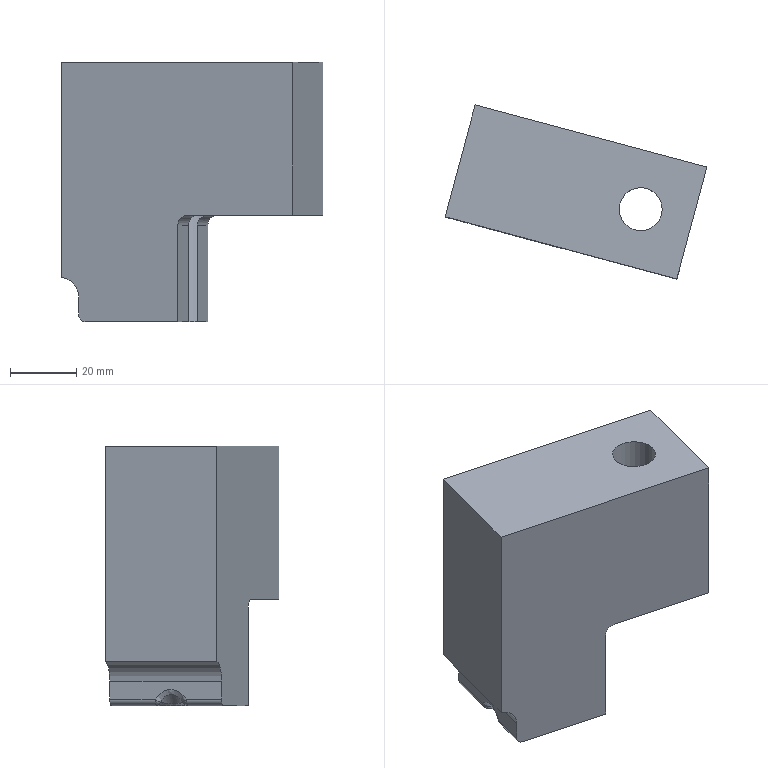Part | NX | features solid 2 | 1 solid | 27 faces | box 79.088 x 52.572 x 78.4 mm | volume 141118 mm3 | plane 12 | cylinder 10 | spline 4 | cone 1 | commonest cylinder face diameters 4 x2 6 x2 8.5 x1 10 x1 11 x1 12 x1
STEP:
#1=CARTESIAN_POINT('',(1214.961,-8.867,-0.02087));
#2=VERTEX_POINT('',#1);
#3=CARTESIAN_POINT('',(1214.961,-8.867,65.));
#4=VERTEX_POINT('',#3);
#5=CARTESIAN_POINT('',(1214.961,-8.867,86.));
#6=DIRECTION('',(0.,0.,1.));
#7=VECTOR('',#6,1000.);
#8=LINE('',#5,#7);
#9=EDGE_CURVE('',#2,#4,#8,.T.);
#10=ORIENTED_EDGE('',*,*,#9,.T.);
#11=CARTESIAN_POINT('',(1284.991,-27.632,65.));
#12=VERTEX_POINT('',#11);
#13=CARTESIAN_POINT('',(1303.344,-32.549,65.));
#14=DIRECTION('',(0.9659,-0.2588,0.));
#15=VECTOR('',#14,1000.);
#16=LINE('',#13,#15);
#17=EDGE_CURVE('',#4,#12,#16,.T.);
#18=ORIENTED_EDGE('',*,*,#17,.T.);
#19=CARTESIAN_POINT('',(1284.991,-27.632,18.75));
#20=VERTEX_POINT('',#19);
#21=CARTESIAN_POINT('',(1284.991,-27.632,142.6));
#22=DIRECTION('',(0.,0.,1.));
#23=VECTOR('',#22,1000.);
#24=LINE('',#21,#23);
#25=EDGE_CURVE('',#20,#12,#24,.T.);
#26=ORIENTED_EDGE('',*,*,#25,.F.);
#27=CARTESIAN_POINT('',(1253.115,-19.091,18.75));
#28=VERTEX_POINT('',#27);
#29=CARTESIAN_POINT('',(1303.344,-32.549,18.75));
#30=DIRECTION('',(0.9659,-0.2588,0.));
#31=VECTOR('',#30,1000.);
#32=LINE('',#29,#31);
#33=EDGE_CURVE('',#20,#28,#32,.F.);
#34=ORIENTED_EDGE('',*,*,#33,.T.);
#35=CARTESIAN_POINT('',(1250.218,-18.314,15.75));
#36=VERTEX_POINT('',#35);
#37=CARTESIAN_POINT('',(1253.115,-19.091,15.75));
#38=DIRECTION('',(-0.2588,-0.9659,0.));
#39=DIRECTION('',(0.9659,-0.2588,0.));
#40=AXIS2_PLACEMENT_3D('',#37,#38,#39);
#41=CIRCLE('',#40,3.);
#42=EDGE_CURVE('',#36,#28,#41,.F.);
#43=ORIENTED_EDGE('',*,*,#42,.F.);
#44=CARTESIAN_POINT('',(1250.218,-18.314,-13.4));
#45=VERTEX_POINT('',#44);
#46=CARTESIAN_POINT('',(1250.218,-18.314,142.6));
#47=DIRECTION('',(0.,0.,1.));
#48=VECTOR('',#47,1000.);
#49=LINE('',#46,#48);
#50=EDGE_CURVE('',#45,#36,#49,.T.);
#51=ORIENTED_EDGE('',*,*,#50,.F.);
#52=CARTESIAN_POINT('',(1222.206,-10.808,-13.4));
#53=VERTEX_POINT('',#52);
#54=CARTESIAN_POINT('',(1303.344,-32.549,-13.4));
#55=DIRECTION('',(0.9659,-0.2588,0.));
#56=VECTOR('',#55,1000.);
#57=LINE('',#54,#56);
#58=EDGE_CURVE('',#45,#53,#57,.F.);
#59=ORIENTED_EDGE('',*,*,#58,.T.);
#60=CARTESIAN_POINT('',(1220.274,-10.291,-11.4));
#61=VERTEX_POINT('',#60);
#62=CARTESIAN_POINT('',(1222.206,-10.808,-11.4));
#63=DIRECTION('',(0.2588,0.9659,0.));
#64=DIRECTION('',(-0.9659,0.2588,0.));
#65=AXIS2_PLACEMENT_3D('',#62,#63,#64);
#66=CIRCLE('',#65,2.);
#67=EDGE_CURVE('',#61,#53,#66,.F.);
#68=ORIENTED_EDGE('',*,*,#67,.F.);
#69=CARTESIAN_POINT('',(1220.274,-10.291,-6.));
#70=VERTEX_POINT('',#69);
#71=CARTESIAN_POINT('',(1220.274,-10.291,0.));
#72=DIRECTION('',(0.,0.,1.));
#73=VECTOR('',#72,1000.);
#74=LINE('',#71,#73);
#75=EDGE_CURVE('',#70,#61,#74,.F.);
#76=ORIENTED_EDGE('',*,*,#75,.F.);
#77=CARTESIAN_POINT('',(1214.478,-8.738,-6.));
#78=DIRECTION('',(0.2588,0.9659,0.));
#79=DIRECTION('',(-0.9659,0.2588,0.));
#80=AXIS2_PLACEMENT_3D('',#77,#78,#79);
#81=CIRCLE('',#80,6.);
#82=EDGE_CURVE('',#2,#70,#81,.T.);
#83=ORIENTED_EDGE('',*,*,#82,.F.);
#84=EDGE_LOOP('',(#10,#18,#26,#34,#43,#51,#59,#68,#76,#83));
#85=FACE_BOUND('',#84,.T.);
#86=CARTESIAN_POINT('',(1303.344,-32.549,-6.));
#87=DIRECTION('',(0.2588,0.9659,0.));
#88=DIRECTION('',(-0.9659,0.2588,0.));
#89=AXIS2_PLACEMENT_3D('',#86,#87,#88);
#90=PLANE('',#89);
#91=ADVANCED_FACE('',(#85),#90,.T.);
#92=CARTESIAN_POINT('',(1205.903,-42.675,65.));
#93=VERTEX_POINT('',#92);
#94=CARTESIAN_POINT('',(1205.903,-42.675,-0.02087));
#95=VERTEX_POINT('',#94);
#96=CARTESIAN_POINT('',(1205.903,-42.675,181.6));
#97=DIRECTION('',(0.,0.,-1.));
#98=VECTOR('',#97,1000.);
#99=LINE('',#96,#98);
#100=EDGE_CURVE('',#93,#95,#99,.T.);
#101=ORIENTED_EDGE('',*,*,#100,.F.);
#102=CARTESIAN_POINT('',(1203.025,-53.415,65.));
#103=DIRECTION('',(0.2588,0.9659,0.));
#104=VECTOR('',#103,1000.);
#105=LINE('',#102,#104);
#106=EDGE_CURVE('',#93,#4,#105,.T.);
#107=ORIENTED_EDGE('',*,*,#106,.T.);
#108=ORIENTED_EDGE('',*,*,#9,.F.);
#109=CARTESIAN_POINT('',(1215.168,-8.097,-0.02087));
#110=DIRECTION('',(0.2588,0.9659,0.));
#111=VECTOR('',#110,1000.);
#112=LINE('',#109,#111);
#113=EDGE_CURVE('',#2,#95,#112,.F.);
#114=ORIENTED_EDGE('',*,*,#113,.T.);
#115=EDGE_LOOP('',(#101,#107,#108,#114));
#116=FACE_BOUND('',#115,.T.);
#117=CARTESIAN_POINT('',(1203.025,-53.415,86.));
#118=DIRECTION('',(-0.9659,0.2588,0.));
#119=DIRECTION('',(-0.2588,-0.9659,0.));
#120=AXIS2_PLACEMENT_3D('',#117,#118,#119);
#121=PLANE('',#120);
#122=ADVANCED_FACE('',(#116),#121,.T.);
#123=CARTESIAN_POINT('',(1275.932,-61.439,65.));
#124=VERTEX_POINT('',#123);
#125=CARTESIAN_POINT('',(1213.147,-44.616,65.));
#126=DIRECTION('',(0.9659,-0.2588,0.));
#127=VECTOR('',#126,1000.);
#128=LINE('',#125,#127);
#129=EDGE_CURVE('',#93,#124,#128,.T.);
#130=ORIENTED_EDGE('',*,*,#129,.F.);
#131=ORIENTED_EDGE('',*,*,#100,.T.);
#132=CARTESIAN_POINT('',(1211.215,-44.098,-6.));
#133=VERTEX_POINT('',#132);
#134=CARTESIAN_POINT('',(1205.42,-42.545,-6.));
#135=DIRECTION('',(0.2588,0.9659,0.));
#136=DIRECTION('',(-0.9659,0.2588,0.));
#137=AXIS2_PLACEMENT_3D('',#134,#135,#136);
#138=CIRCLE('',#137,6.);
#139=EDGE_CURVE('',#133,#95,#138,.F.);
#140=ORIENTED_EDGE('',*,*,#139,.F.);
#141=CARTESIAN_POINT('',(1211.215,-44.098,-11.4));
#142=VERTEX_POINT('',#141);
#143=CARTESIAN_POINT('',(1211.215,-44.098,0.));
#144=DIRECTION('',(0.,0.,1.));
#145=VECTOR('',#144,1000.);
#146=LINE('',#143,#145);
#147=EDGE_CURVE('',#142,#133,#146,.T.);
#148=ORIENTED_EDGE('',*,*,#147,.F.);
#149=CARTESIAN_POINT('',(1213.147,-44.616,-13.4));
#150=VERTEX_POINT('',#149);
#151=CARTESIAN_POINT('',(1213.147,-44.616,-11.4));
#152=DIRECTION('',(0.2588,0.9659,0.));
#153=DIRECTION('',(-0.9659,0.2588,0.));
#154=AXIS2_PLACEMENT_3D('',#151,#152,#153);
#155=CIRCLE('',#154,2.);
#156=EDGE_CURVE('',#142,#150,#155,.F.);
#157=ORIENTED_EDGE('',*,*,#156,.T.);
#158=CARTESIAN_POINT('',(1241.159,-52.122,-13.4));
#159=VERTEX_POINT('',#158);
#160=CARTESIAN_POINT('',(1211.215,-44.098,-13.4));
#161=DIRECTION('',(-0.9659,0.2588,0.));
#162=VECTOR('',#161,1000.);
#163=LINE('',#160,#162);
#164=EDGE_CURVE('',#159,#150,#163,.T.);
#165=ORIENTED_EDGE('',*,*,#164,.F.);
#166=CARTESIAN_POINT('',(1241.159,-52.122,15.75));
#167=VERTEX_POINT('',#166);
#168=CARTESIAN_POINT('',(1241.159,-52.122,142.6));
#169=DIRECTION('',(0.,0.,1.));
#170=VECTOR('',#169,1000.);
#171=LINE('',#168,#170);
#172=EDGE_CURVE('',#159,#167,#171,.T.);
#173=ORIENTED_EDGE('',*,*,#172,.T.);
#174=CARTESIAN_POINT('',(1244.057,-52.898,18.75));
#175=VERTEX_POINT('',#174);
#176=CARTESIAN_POINT('',(1244.057,-52.898,15.75));
#177=DIRECTION('',(-0.2588,-0.9659,0.));
#178=DIRECTION('',(0.9659,-0.2588,0.));
#179=AXIS2_PLACEMENT_3D('',#176,#177,#178);
#180=CIRCLE('',#179,3.);
#181=EDGE_CURVE('',#175,#167,#180,.T.);
#182=ORIENTED_EDGE('',*,*,#181,.F.);
#183=CARTESIAN_POINT('',(1275.932,-61.439,18.75));
#184=VERTEX_POINT('',#183);
#185=CARTESIAN_POINT('',(1213.147,-44.616,18.75));
#186=DIRECTION('',(0.9659,-0.2588,0.));
#187=VECTOR('',#186,1000.);
#188=LINE('',#185,#187);
#189=EDGE_CURVE('',#184,#175,#188,.F.);
#190=ORIENTED_EDGE('',*,*,#189,.F.);
#191=CARTESIAN_POINT('',(1275.932,-61.439,142.6));
#192=DIRECTION('',(0.,0.,1.));
#193=VECTOR('',#192,1000.);
#194=LINE('',#191,#193);
#195=EDGE_CURVE('',#184,#124,#194,.T.);
#196=ORIENTED_EDGE('',*,*,#195,.T.);
#197=EDGE_LOOP('',(#130,#131,#140,#148,#157,#165,#173,#182,#190,#196));
#198=FACE_BOUND('',#197,.T.);
#199=CARTESIAN_POINT('',(1213.147,-44.616,181.6));
#200=DIRECTION('',(0.2588,0.9659,0.));
#201=DIRECTION('',(-0.9659,0.2588,0.));
#202=AXIS2_PLACEMENT_3D('',#199,#200,#201);
#203=PLANE('',#202);
#204=ADVANCED_FACE('',(#198),#203,.F.);
#205=ORIENTED_EDGE('',*,*,#25,.T.);
#206=CARTESIAN_POINT('',(1285.197,-26.861,65.));
#207=DIRECTION('',(-0.2588,-0.9659,0.));
#208=VECTOR('',#207,1000.);
#209=LINE('',#206,#208);
#210=EDGE_CURVE('',#12,#124,#209,.T.);
#211=ORIENTED_EDGE('',*,*,#210,.T.);
#212=ORIENTED_EDGE('',*,*,#195,.F.);
#213=CARTESIAN_POINT('',(1245.599,-174.645,18.75));
#214=DIRECTION('',(-0.2588,-0.9659,0.));
#215=VECTOR('',#214,1000.);
#216=LINE('',#213,#215);
#217=EDGE_CURVE('',#184,#20,#216,.F.);
#218=ORIENTED_EDGE('',*,*,#217,.T.);
#219=EDGE_LOOP('',(#205,#211,#212,#218));
#220=FACE_BOUND('',#219,.T.);
#221=CARTESIAN_POINT('',(1285.197,-26.861,142.6));
#222=DIRECTION('',(0.9659,-0.2588,0.));
#223=DIRECTION('',(0.2588,0.9659,0.));
#224=AXIS2_PLACEMENT_3D('',#221,#222,#223);
#225=PLANE('',#224);
#226=ADVANCED_FACE('',(#220),#225,.T.);
#227=CARTESIAN_POINT('',(1271.507,-40.394,48.));
#228=VERTEX_POINT('',#227);
#229=CARTESIAN_POINT('',(1265.007,-40.394,48.));
#230=DIRECTION('',(0.,0.,-1.));
#231=DIRECTION('',(1.,0.,0.));
#232=AXIS2_PLACEMENT_3D('',#229,#230,#231);
#233=CIRCLE('',#232,6.5);
#234=EDGE_CURVE('',#228,#228,#233,.F.);
#235=ORIENTED_EDGE('',*,*,#234,.F.);
#236=EDGE_LOOP('',(#235));
#237=FACE_BOUND('',#236,.T.);
#238=CARTESIAN_POINT('',(1271.507,-40.394,65.));
#239=VERTEX_POINT('',#238);
#240=CARTESIAN_POINT('',(1265.007,-40.394,65.));
#241=DIRECTION('',(0.,0.,1.));
#242=DIRECTION('',(1.,0.,0.));
#243=AXIS2_PLACEMENT_3D('',#240,#241,#242);
#244=CIRCLE('',#243,6.5);
#245=EDGE_CURVE('',#239,#239,#244,.F.);
#246=ORIENTED_EDGE('',*,*,#245,.F.);
#247=EDGE_LOOP('',(#246));
#248=FACE_BOUND('',#247,.T.);
#249=CARTESIAN_POINT('',(1265.007,-40.394,53.75));
#250=DIRECTION('',(0.,0.,1.));
#251=DIRECTION('',(1.,0.,0.));
#252=AXIS2_PLACEMENT_3D('',#249,#250,#251);
#253=CYLINDRICAL_SURFACE('',#252,6.5);
#254=ADVANCED_FACE('',(#237,#248),#253,.F.);
#255=CARTESIAN_POINT('',(1247.014,-30.269,15.75));
#256=VERTEX_POINT('',#255);
#257=CARTESIAN_POINT('',(1247.014,-30.269,-13.4));
#258=VERTEX_POINT('',#257);
#259=CARTESIAN_POINT('',(1247.014,-30.269,18.75));
#260=DIRECTION('',(0.,0.,-1.));
#261=VECTOR('',#260,1000.);
#262=LINE('',#259,#261);
#263=EDGE_CURVE('',#256,#258,#262,.T.);
#264=ORIENTED_EDGE('',*,*,#263,.T.);
#265=CARTESIAN_POINT('',(1242.3,-47.861,-13.4));
#266=DIRECTION('',(0.2588,0.9659,0.));
#267=VECTOR('',#266,1000.);
#268=LINE('',#265,#267);
#269=EDGE_CURVE('',#258,#45,#268,.T.);
#270=ORIENTED_EDGE('',*,*,#269,.T.);
#271=ORIENTED_EDGE('',*,*,#50,.T.);
#272=CARTESIAN_POINT('',(1250.424,-17.544,15.75));
#273=DIRECTION('',(-0.2588,-0.9659,0.));
#274=VECTOR('',#273,1000.);
#275=LINE('',#272,#274);
#276=EDGE_CURVE('',#256,#36,#275,.F.);
#277=ORIENTED_EDGE('',*,*,#276,.F.);
#278=EDGE_LOOP('',(#264,#270,#271,#277));
#279=FACE_BOUND('',#278,.T.);
#280=CARTESIAN_POINT('',(1250.424,-17.544,142.6));
#281=DIRECTION('',(0.9659,-0.2588,0.));
#282=DIRECTION('',(0.2588,0.9659,0.));
#283=AXIS2_PLACEMENT_3D('',#280,#281,#282);
#284=PLANE('',#283);
#285=ADVANCED_FACE('',(#279),#284,.T.);
#286=ORIENTED_EDGE('',*,*,#172,.F.);
#287=CARTESIAN_POINT('',(1244.362,-40.167,-13.4));
#288=VERTEX_POINT('',#287);
#289=CARTESIAN_POINT('',(1242.3,-47.861,-13.4));
#290=DIRECTION('',(0.2588,0.9659,0.));
#291=VECTOR('',#290,1000.);
#292=LINE('',#289,#291);
#293=EDGE_CURVE('',#159,#288,#292,.T.);
#294=ORIENTED_EDGE('',*,*,#293,.T.);
#295=CARTESIAN_POINT('',(1244.362,-40.167,15.75));
#296=VERTEX_POINT('',#295);
#297=CARTESIAN_POINT('',(1244.362,-40.167,-13.4));
#298=DIRECTION('',(0.,0.,-1.));
#299=VECTOR('',#298,1000.);
#300=LINE('',#297,#299);
#301=EDGE_CURVE('',#288,#296,#300,.F.);
#302=ORIENTED_EDGE('',*,*,#301,.T.);
#303=CARTESIAN_POINT('',(1250.424,-17.544,15.75));
#304=DIRECTION('',(-0.2588,-0.9659,0.));
#305=VECTOR('',#304,1000.);
#306=LINE('',#303,#305);
#307=EDGE_CURVE('',#167,#296,#306,.F.);
#308=ORIENTED_EDGE('',*,*,#307,.F.);
#309=EDGE_LOOP('',(#286,#294,#302,#308));
#310=FACE_BOUND('',#309,.T.);
#311=CARTESIAN_POINT('',(1250.424,-17.544,142.6));
#312=DIRECTION('',(0.9659,-0.2588,0.));
#313=DIRECTION('',(0.2588,0.9659,0.));
#314=AXIS2_PLACEMENT_3D('',#311,#312,#313);
#315=PLANE('',#314);
#316=ADVANCED_FACE('',(#310),#315,.T.);
#317=CARTESIAN_POINT('',(1217.195,-25.606,-12.41));
#318=VERTEX_POINT('',#317);
#319=CARTESIAN_POINT('',(1216.601,-23.998,-11.4));
#320=VERTEX_POINT('',#319);
#321=CARTESIAN_POINT('',(1217.195,-25.606,-12.41));
#322=CARTESIAN_POINT('',(1217.092,-25.518,-12.368));
#323=CARTESIAN_POINT('',(1216.836,-25.249,-12.228));
#324=CARTESIAN_POINT('',(1216.559,-24.723,-11.913));
#325=CARTESIAN_POINT('',(1216.534,-24.249,-11.588));
#326=CARTESIAN_POINT('',(1216.601,-23.998,-11.4));
#327=B_SPLINE_CURVE_WITH_KNOTS('',3,(#321,#322,#323,#324,#325,#326),.UNSPECIFIED.,.F.,.F.,(4,1,1,4),(0.,0.25,0.5,1.),.UNSPECIFIED.);
#328=EDGE_CURVE('',#318,#320,#327,.T.);
#329=ORIENTED_EDGE('',*,*,#328,.T.);
#330=CARTESIAN_POINT('',(1218.533,-24.515,-13.4));
#331=VERTEX_POINT('',#330);
#332=CARTESIAN_POINT('',(1218.533,-24.515,-11.4));
#333=DIRECTION('',(-0.2588,-0.9659,0.));
#334=DIRECTION('',(-0.9659,0.2588,0.));
#335=AXIS2_PLACEMENT_3D('',#332,#333,#334);
#336=CIRCLE('',#335,2.);
#337=EDGE_CURVE('',#331,#320,#336,.F.);
#338=ORIENTED_EDGE('',*,*,#337,.F.);
#339=CARTESIAN_POINT('',(1218.533,-24.515,-13.4));
#340=CARTESIAN_POINT('',(1218.423,-24.605,-13.4));
#341=CARTESIAN_POINT('',(1218.117,-24.854,-13.353));
#342=CARTESIAN_POINT('',(1217.758,-25.147,-13.159));
#343=CARTESIAN_POINT('',(1217.421,-25.422,-12.819));
#344=CARTESIAN_POINT('',(1217.28,-25.537,-12.597));
#345=CARTESIAN_POINT('',(1217.195,-25.606,-12.41));
#346=B_SPLINE_CURVE_WITH_KNOTS('',3,(#339,#340,#341,#342,#343,#344,#345),.UNSPECIFIED.,.F.,.F.,(4,1,1,1,4),(0.,0.25,0.5,0.75,1.),.UNSPECIFIED.);
#347=EDGE_CURVE('',#318,#331,#346,.F.);
#348=ORIENTED_EDGE('',*,*,#347,.F.);
#349=EDGE_LOOP('',(#329,#338,#348));
#350=FACE_BOUND('',#349,.T.);
#351=CARTESIAN_POINT('',(1218.548,-23.887,-13.299));
#352=CARTESIAN_POINT('',(1218.458,-24.219,-13.409));
#353=CARTESIAN_POINT('',(1218.515,-24.574,-13.431));
#354=CARTESIAN_POINT('',(1218.706,-24.871,-13.36));
#355=CARTESIAN_POINT('',(1217.473,-23.62,-13.219));
#356=CARTESIAN_POINT('',(1217.302,-24.242,-13.426));
#357=CARTESIAN_POINT('',(1217.41,-24.91,-13.468));
#358=CARTESIAN_POINT('',(1217.77,-25.469,-13.335));
#359=CARTESIAN_POINT('',(1216.682,-23.663,-12.44));
#360=CARTESIAN_POINT('',(1216.488,-24.372,-12.676));
#361=CARTESIAN_POINT('',(1216.61,-25.134,-12.723));
#362=CARTESIAN_POINT('',(1217.021,-25.77,-12.571));
#363=CARTESIAN_POINT('',(1216.602,-23.993,-11.382));
#364=CARTESIAN_POINT('',(1216.453,-24.538,-11.563));
#365=CARTESIAN_POINT('',(1216.547,-25.123,-11.6));
#366=CARTESIAN_POINT('',(1216.863,-25.612,-11.483));
#367=(BOUNDED_SURFACE()B_SPLINE_SURFACE(3,3,((#351,#352,#353,#354),(#355,#356,#357,#358),(#359,#360,#361,#362),(#363,#364,#365,#366)),.UNSPECIFIED.,.F.,.F.,.F.)B_SPLINE_SURFACE_WITH_KNOTS((4,4),(4,4),(0.0005941,0.9994),(0.000239,0.9998),.PIECEWISE_BEZIER_KNOTS.)GEOMETRIC_REPRESENTATION_ITEM()RATIONAL_B_SPLINE_SURFACE(((0.9996,0.9224,0.9224,0.9996),(0.8197,0.7563,0.7563,0.8197),(0.8197,0.7563,0.7563,0.8197),(0.9996,0.9224,0.9224,0.9996)))REPRESENTATION_ITEM('')SURFACE());
#368=ADVANCED_FACE('',(#350),#367,.F.);
#369=CARTESIAN_POINT('',(1218.631,-29.613,-12.814));
#370=VERTEX_POINT('',#369);
#371=CARTESIAN_POINT('',(1217.195,-25.606,-12.41));
#372=CARTESIAN_POINT('',(1217.496,-25.918,-12.472));
#373=CARTESIAN_POINT('',(1218.01,-26.568,-12.582));
#374=CARTESIAN_POINT('',(1218.487,-27.429,-12.697));
#375=CARTESIAN_POINT('',(1218.791,-28.607,-12.796));
#376=CARTESIAN_POINT('',(1218.719,-29.284,-12.814));
#377=CARTESIAN_POINT('',(1218.631,-29.613,-12.814));
#378=B_SPLINE_CURVE_WITH_KNOTS('',3,(#371,#372,#373,#374,#375,#376,#377),.UNSPECIFIED.,.F.,.F.,(4,1,1,1,4),(0.000000039,0.25,0.5,0.75,1.),.UNSPECIFIED.);
#379=EDGE_CURVE('',#370,#318,#378,.F.);
#380=ORIENTED_EDGE('',*,*,#379,.F.);
#381=CARTESIAN_POINT('',(1215.384,-32.366,-12.41));
#382=VERTEX_POINT('',#381);
#383=CARTESIAN_POINT('',(1218.631,-29.613,-12.814));
#384=CARTESIAN_POINT('',(1218.543,-29.942,-12.814));
#385=CARTESIAN_POINT('',(1218.266,-30.564,-12.796));
#386=CARTESIAN_POINT('',(1217.414,-31.433,-12.697));
#387=CARTESIAN_POINT('',(1216.571,-31.94,-12.582));
#388=CARTESIAN_POINT('',(1215.801,-32.246,-12.472));
#389=CARTESIAN_POINT('',(1215.384,-32.366,-12.41));
#390=B_SPLINE_CURVE_WITH_KNOTS('',3,(#383,#384,#385,#386,#387,#388,#389),.UNSPECIFIED.,.F.,.F.,(4,1,1,1,4),(0.,0.25,0.5,0.75,1.),.UNSPECIFIED.);
#391=EDGE_CURVE('',#382,#370,#390,.F.);
#392=ORIENTED_EDGE('',*,*,#391,.F.);
#393=CARTESIAN_POINT('',(1215.899,-28.881,-9.986));
#394=VERTEX_POINT('',#393);
#395=CARTESIAN_POINT('',(1215.899,-28.881,-9.986));
#396=CARTESIAN_POINT('',(1215.716,-29.563,-9.986));
#397=CARTESIAN_POINT('',(1215.439,-30.969,-10.562));
#398=CARTESIAN_POINT('',(1215.38,-31.927,-11.708));
#399=CARTESIAN_POINT('',(1215.384,-32.366,-12.41));
#400=B_SPLINE_CURVE_WITH_KNOTS('',3,(#395,#396,#397,#398,#399),.UNSPECIFIED.,.F.,.F.,(4,1,4),(0.,0.5,1.),.UNSPECIFIED.);
#401=EDGE_CURVE('',#382,#394,#400,.F.);
#402=ORIENTED_EDGE('',*,*,#401,.T.);
#403=CARTESIAN_POINT('',(1215.899,-28.881,-9.986));
#404=CARTESIAN_POINT('',(1215.99,-28.54,-9.986));
#405=CARTESIAN_POINT('',(1216.196,-27.854,-10.113));
#406=CARTESIAN_POINT('',(1216.544,-26.924,-10.685));
#407=CARTESIAN_POINT('',(1216.844,-26.251,-11.376));
#408=CARTESIAN_POINT('',(1217.077,-25.806,-12.039));
#409=CARTESIAN_POINT('',(1217.195,-25.606,-12.41));
#410=B_SPLINE_CURVE_WITH_KNOTS('',3,(#403,#404,#405,#406,#407,#408,#409),.UNSPECIFIED.,.F.,.F.,(4,1,1,1,4),(0.,0.25,0.5,0.75,1.),.UNSPECIFIED.);
#411=EDGE_CURVE('',#394,#318,#410,.T.);
#412=ORIENTED_EDGE('',*,*,#411,.T.);
#413=EDGE_LOOP('',(#380,#392,#402,#412));
#414=FACE_BOUND('',#413,.T.);
#415=CARTESIAN_POINT('',(1213.815,-28.323,-14.899));
#416=DIRECTION('',(-0.683,0.183,0.7071));
#417=DIRECTION('',(-0.683,0.183,-0.7071));
#418=AXIS2_PLACEMENT_3D('',#415,#416,#417);
#419=CYLINDRICAL_SURFACE('',#418,5.);
#420=ADVANCED_FACE('',(#414),#419,.F.);
#421=CARTESIAN_POINT('',(1214.065,-33.462,-11.4));
#422=VERTEX_POINT('',#421);
#423=CARTESIAN_POINT('',(1214.065,-33.462,-11.4));
#424=CARTESIAN_POINT('',(1214.095,-33.351,-11.483));
#425=CARTESIAN_POINT('',(1214.223,-33.054,-11.714));
#426=CARTESIAN_POINT('',(1214.507,-32.741,-11.985));
#427=CARTESIAN_POINT('',(1214.927,-32.488,-12.24));
#428=CARTESIAN_POINT('',(1215.18,-32.403,-12.346));
#429=CARTESIAN_POINT('',(1215.384,-32.366,-12.41));
#430=B_SPLINE_CURVE_WITH_KNOTS('',3,(#423,#424,#425,#426,#427,#428,#429),.UNSPECIFIED.,.F.,.F.,(4,1,1,1,4),(0.,0.25,0.5,0.75,1.),.UNSPECIFIED.);
#431=EDGE_CURVE('',#422,#382,#430,.T.);
#432=ORIENTED_EDGE('',*,*,#431,.T.);
#433=CARTESIAN_POINT('',(1215.997,-33.979,-13.4));
#434=VERTEX_POINT('',#433);
#435=CARTESIAN_POINT('',(1215.384,-32.366,-12.41));
#436=CARTESIAN_POINT('',(1215.409,-32.432,-12.532));
#437=CARTESIAN_POINT('',(1215.494,-32.656,-12.849));
#438=CARTESIAN_POINT('',(1215.685,-33.159,-13.253));
#439=CARTESIAN_POINT('',(1215.883,-33.679,-13.4));
#440=CARTESIAN_POINT('',(1215.997,-33.979,-13.4));
#441=B_SPLINE_CURVE_WITH_KNOTS('',3,(#435,#436,#437,#438,#439,#440),.UNSPECIFIED.,.F.,.F.,(4,1,1,4),(0.,0.25,0.5,1.),.UNSPECIFIED.);
#442=EDGE_CURVE('',#434,#382,#441,.F.);
#443=ORIENTED_EDGE('',*,*,#442,.F.);
#444=CARTESIAN_POINT('',(1215.997,-33.979,-11.4));
#445=DIRECTION('',(0.2588,0.9659,0.));
#446=DIRECTION('',(-0.9659,0.2588,0.));
#447=AXIS2_PLACEMENT_3D('',#444,#445,#446);
#448=CIRCLE('',#447,2.);
#449=EDGE_CURVE('',#422,#434,#448,.F.);
#450=ORIENTED_EDGE('',*,*,#449,.F.);
#451=EDGE_LOOP('',(#432,#443,#450));
#452=FACE_BOUND('',#451,.T.);
#453=CARTESIAN_POINT('',(1214.005,-34.078,-11.546));
#454=CARTESIAN_POINT('',(1213.987,-33.718,-11.548));
#455=CARTESIAN_POINT('',(1214.051,-33.395,-11.401));
#456=CARTESIAN_POINT('',(1214.181,-33.184,-11.139));
#457=CARTESIAN_POINT('',(1214.086,-34.079,-12.656));
#458=CARTESIAN_POINT('',(1214.053,-33.402,-12.659));
#459=CARTESIAN_POINT('',(1214.173,-32.794,-12.383));
#460=CARTESIAN_POINT('',(1214.417,-32.397,-11.89));
#461=CARTESIAN_POINT('',(1214.904,-34.043,-13.41));
#462=CARTESIAN_POINT('',(1214.866,-33.271,-13.414));
#463=CARTESIAN_POINT('',(1215.002,-32.578,-13.098));
#464=CARTESIAN_POINT('',(1215.281,-32.126,-12.536));
#465=CARTESIAN_POINT('',(1216.015,-33.989,-13.4));
#466=CARTESIAN_POINT('',(1215.986,-33.396,-13.403));
#467=CARTESIAN_POINT('',(1216.091,-32.864,-13.161));
#468=CARTESIAN_POINT('',(1216.305,-32.517,-12.729));
#469=(BOUNDED_SURFACE()B_SPLINE_SURFACE(3,3,((#453,#454,#455,#456),(#457,#458,#459,#460),(#461,#462,#463,#464),(#465,#466,#467,#468)),.UNSPECIFIED.,.F.,.F.,.F.)B_SPLINE_SURFACE_WITH_KNOTS((4,4),(4,4),(0.,1.),(0.,1.),.PIECEWISE_BEZIER_KNOTS.)GEOMETRIC_REPRESENTATION_ITEM()RATIONAL_B_SPLINE_SURFACE(((1.,0.9226,0.9226,1.),(0.8196,0.7562,0.7562,0.8196),(0.8196,0.7562,0.7562,0.8196),(1.,0.9226,0.9226,1.)))REPRESENTATION_ITEM('')SURFACE());
#470=ADVANCED_FACE('',(#452),#469,.F.);
#471=ORIENTED_EDGE('',*,*,#431,.F.);
#472=CARTESIAN_POINT('',(1214.065,-33.462,-11.4));
#473=CARTESIAN_POINT('',(1214.141,-33.181,-10.997));
#474=CARTESIAN_POINT('',(1214.303,-32.574,-10.273));
#475=CARTESIAN_POINT('',(1214.581,-31.538,-9.387));
#476=CARTESIAN_POINT('',(1214.975,-30.067,-8.69));
#477=CARTESIAN_POINT('',(1215.325,-28.758,-8.504));
#478=CARTESIAN_POINT('',(1215.724,-27.272,-8.723));
#479=CARTESIAN_POINT('',(1216.189,-25.536,-9.585));
#480=CARTESIAN_POINT('',(1216.451,-24.557,-10.597));
#481=CARTESIAN_POINT('',(1216.601,-23.998,-11.4));
#482=B_SPLINE_CURVE_WITH_KNOTS('',3,(#472,#473,#474,#475,#476,#477,#478,#479,#480,#481),.UNSPECIFIED.,.F.,.F.,(4,1,1,1,1,1,1,4),(0.,0.125,0.25,0.375,0.5,0.625,0.75,1.),.UNSPECIFIED.);
#483=EDGE_CURVE('',#320,#422,#482,.F.);
#484=ORIENTED_EDGE('',*,*,#483,.F.);
#485=ORIENTED_EDGE('',*,*,#328,.F.);
#486=ORIENTED_EDGE('',*,*,#411,.F.);
#487=ORIENTED_EDGE('',*,*,#401,.F.);
#488=EDGE_LOOP('',(#471,#484,#485,#486,#487));
#489=FACE_BOUND('',#488,.T.);
#490=CARTESIAN_POINT('',(1217.213,-25.576,-12.466));
#491=CARTESIAN_POINT('',(1216.369,-24.862,-12.132));
#492=CARTESIAN_POINT('',(1216.613,-23.952,-11.464));
#493=CARTESIAN_POINT('',(1216.721,-26.403,-10.898));
#494=CARTESIAN_POINT('',(1216.13,-25.757,-10.49));
#495=CARTESIAN_POINT('',(1216.278,-25.204,-9.636));
#496=CARTESIAN_POINT('',(1215.752,-28.842,-9.074));
#497=CARTESIAN_POINT('',(1215.333,-28.73,-8.356));
#498=CARTESIAN_POINT('',(1215.333,-28.73,-7.507));
#499=CARTESIAN_POINT('',(1215.372,-31.439,-10.898));
#500=CARTESIAN_POINT('',(1214.537,-31.702,-10.49));
#501=CARTESIAN_POINT('',(1214.388,-32.255,-9.636));
#502=CARTESIAN_POINT('',(1215.384,-32.4,-12.466));
#503=CARTESIAN_POINT('',(1214.297,-32.597,-12.132));
#504=CARTESIAN_POINT('',(1214.053,-33.507,-11.464));
#505=(BOUNDED_SURFACE()B_SPLINE_SURFACE(3,2,((#490,#491,#492),(#493,#494,#495),(#496,#497,#498),(#499,#500,#501),(#502,#503,#504)),.UNSPECIFIED.,.F.,.F.,.F.)B_SPLINE_SURFACE_WITH_KNOTS((4,1,4),(3,3),(5.499,6.283,7.068),(0.,1.),.UNSPECIFIED.)GEOMETRIC_REPRESENTATION_ITEM()RATIONAL_B_SPLINE_SURFACE(((1.,0.8662,1.),(1.,0.9039,1.),(1.,0.9439,1.),(1.,0.9039,1.),(1.,0.8662,1.)))REPRESENTATION_ITEM('')SURFACE());
#506=ADVANCED_FACE('',(#489),#505,.T.);
#507=CARTESIAN_POINT('',(1215.255,-36.748,-13.4));
#508=DIRECTION('',(0.2588,0.9659,0.));
#509=VECTOR('',#508,1000.);
#510=LINE('',#507,#509);
#511=EDGE_CURVE('',#331,#53,#510,.T.);
#512=ORIENTED_EDGE('',*,*,#511,.F.);
#513=ORIENTED_EDGE('',*,*,#337,.T.);
#514=CARTESIAN_POINT('',(1208.337,-54.839,-11.4));
#515=DIRECTION('',(-0.2588,-0.9659,0.));
#516=VECTOR('',#515,1000.);
#517=LINE('',#514,#516);
#518=EDGE_CURVE('',#61,#320,#517,.T.);
#519=ORIENTED_EDGE('',*,*,#518,.F.);
#520=ORIENTED_EDGE('',*,*,#67,.T.);
#521=EDGE_LOOP('',(#512,#513,#519,#520));
#522=FACE_BOUND('',#521,.T.);
#523=CARTESIAN_POINT('',(1215.255,-36.748,-11.4));
#524=DIRECTION('',(0.2588,0.9659,0.));
#525=DIRECTION('',(0.9659,-0.2588,0.));
#526=AXIS2_PLACEMENT_3D('',#523,#524,#525);
#527=CYLINDRICAL_SURFACE('',#526,2.);
#528=ADVANCED_FACE('',(#522),#527,.T.);
#529=ORIENTED_EDGE('',*,*,#379,.T.);
#530=ORIENTED_EDGE('',*,*,#347,.T.);
#531=CARTESIAN_POINT('',(1218.533,-24.515,-13.4));
#532=CARTESIAN_POINT('',(1218.674,-24.688,-13.4));
#533=CARTESIAN_POINT('',(1218.87,-24.947,-13.4));
#534=CARTESIAN_POINT('',(1219.116,-25.318,-13.4));
#535=CARTESIAN_POINT('',(1219.262,-25.552,-13.4));
#536=CARTESIAN_POINT('',(1219.491,-25.972,-13.4));
#537=CARTESIAN_POINT('',(1219.642,-26.288,-13.4));
#538=CARTESIAN_POINT('',(1219.872,-26.858,-13.4));
#539=CARTESIAN_POINT('',(1220.033,-27.454,-13.4));
#540=CARTESIAN_POINT('',(1220.082,-27.715,-13.4));
#541=CARTESIAN_POINT('',(1220.153,-28.177,-13.4));
#542=CARTESIAN_POINT('',(1220.191,-28.931,-13.4));
#543=CARTESIAN_POINT('',(1220.078,-29.785,-13.4));
#544=CARTESIAN_POINT('',(1219.84,-30.483,-13.4));
#545=CARTESIAN_POINT('',(1219.676,-30.855,-13.4));
#546=CARTESIAN_POINT('',(1219.506,-31.175,-13.4));
#547=CARTESIAN_POINT('',(1219.427,-31.305,-13.4));
#548=CARTESIAN_POINT('',(1219.318,-31.478,-13.4));
#549=CARTESIAN_POINT('',(1219.195,-31.652,-13.4));
#550=CARTESIAN_POINT('',(1219.117,-31.763,-13.4));
#551=CARTESIAN_POINT('',(1218.836,-32.106,-13.4));
#552=CARTESIAN_POINT('',(1218.584,-32.369,-13.4));
#553=CARTESIAN_POINT('',(1218.287,-32.644,-13.4));
#554=CARTESIAN_POINT('',(1218.013,-32.871,-13.4));
#555=CARTESIAN_POINT('',(1217.557,-33.199,-13.4));
#556=CARTESIAN_POINT('',(1216.981,-33.549,-13.4));
#557=CARTESIAN_POINT('',(1216.389,-33.83,-13.4));
#558=CARTESIAN_POINT('',(1215.997,-33.979,-13.4));
#559=B_SPLINE_CURVE_WITH_KNOTS('',3,(#531,#532,#533,#534,#535,#536,#537,#538,#539,#540,#541,#542,#543,#544,#545,#546,#547,#548,#549,#550,#551,#552,#553,#554,#555,#556,#557,#558),.UNSPECIFIED.,.F.,.F.,(4,1,1,1,1,1,1,1,1,1,1,1,1,1,1,1,1,1,1,1,1,1,1,1,1,4),(0.,0.0625,0.09375,0.125,0.1562,0.1875,0.2188,0.25,0.2812,0.3125,0.375,0.5,0.5625,0.5938,0.625,0.6562,0.6875,0.7188,0.75,0.7812,0.8125,0.8438,0.875,0.9062,0.9375,1.),.UNSPECIFIED.);
#560=EDGE_CURVE('',#434,#331,#559,.F.);
#561=ORIENTED_EDGE('',*,*,#560,.F.);
#562=ORIENTED_EDGE('',*,*,#442,.T.);
#563=ORIENTED_EDGE('',*,*,#391,.T.);
#564=EDGE_LOOP('',(#529,#530,#561,#562,#563));
#565=FACE_BOUND('',#564,.T.);
#566=CARTESIAN_POINT('',(1215.321,-32.383,-12.4));
#567=CARTESIAN_POINT('',(1215.522,-32.925,-13.4));
#568=CARTESIAN_POINT('',(1215.923,-34.008,-13.4));
#569=CARTESIAN_POINT('',(1217.075,-31.895,-12.662));
#570=CARTESIAN_POINT('',(1217.347,-32.455,-13.4));
#571=CARTESIAN_POINT('',(1218.025,-33.23,-13.4));
#572=CARTESIAN_POINT('',(1219.512,-29.849,-12.966));
#573=CARTESIAN_POINT('',(1220.206,-30.035,-13.4));
#574=CARTESIAN_POINT('',(1221.026,-30.255,-13.4));
#575=CARTESIAN_POINT('',(1218.424,-26.859,-12.662));
#576=CARTESIAN_POINT('',(1218.94,-26.51,-13.4));
#577=CARTESIAN_POINT('',(1219.914,-26.178,-13.4));
#578=CARTESIAN_POINT('',(1217.15,-25.56,-12.4));
#579=CARTESIAN_POINT('',(1217.594,-25.191,-13.4));
#580=CARTESIAN_POINT('',(1218.483,-24.453,-13.4));
#581=(BOUNDED_SURFACE()B_SPLINE_SURFACE(3,2,((#566,#567,#568),(#569,#570,#571),(#572,#573,#574),(#575,#576,#577),(#578,#579,#580)),.UNSPECIFIED.,.F.,.F.,.F.)B_SPLINE_SURFACE_WITH_KNOTS((4,1,4),(3,3),(2.357,3.142,3.926),(0.,1.),.UNSPECIFIED.)GEOMETRIC_REPRESENTATION_ITEM()RATIONAL_B_SPLINE_SURFACE(((1.,0.8662,1.),(1.,0.9039,1.),(1.,0.9439,1.),(1.,0.9039,1.),(1.,0.8662,1.)))REPRESENTATION_ITEM('')SURFACE());
#582=ADVANCED_FACE('',(#565),#581,.T.);
#583=CARTESIAN_POINT('',(1204.828,-67.934,-6.));
#584=DIRECTION('',(0.2588,0.9659,0.));
#585=VECTOR('',#584,1000.);
#586=LINE('',#583,#585);
#587=EDGE_CURVE('',#70,#133,#586,.F.);
#588=ORIENTED_EDGE('',*,*,#587,.T.);
#589=ORIENTED_EDGE('',*,*,#139,.T.);
#590=ORIENTED_EDGE('',*,*,#113,.F.);
#591=ORIENTED_EDGE('',*,*,#82,.T.);
#592=EDGE_LOOP('',(#588,#589,#590,#591));
#593=FACE_BOUND('',#592,.T.);
#594=CARTESIAN_POINT('',(1199.033,-66.381,-6.));
#595=DIRECTION('',(0.2588,0.9659,0.));
#596=DIRECTION('',(0.9659,-0.2588,0.));
#597=AXIS2_PLACEMENT_3D('',#594,#595,#596);
#598=CYLINDRICAL_SURFACE('',#597,6.);
#599=ADVANCED_FACE('',(#593),#598,.F.);
#600=ORIENTED_EDGE('',*,*,#293,.F.);
#601=ORIENTED_EDGE('',*,*,#164,.T.);
#602=CARTESIAN_POINT('',(1215.255,-36.748,-13.4));
#603=DIRECTION('',(0.2588,0.9659,0.));
#604=VECTOR('',#603,1000.);
#605=LINE('',#602,#604);
#606=EDGE_CURVE('',#150,#434,#605,.T.);
#607=ORIENTED_EDGE('',*,*,#606,.T.);
#608=ORIENTED_EDGE('',*,*,#560,.T.);
#609=ORIENTED_EDGE('',*,*,#511,.T.);
#610=ORIENTED_EDGE('',*,*,#58,.F.);
#611=ORIENTED_EDGE('',*,*,#269,.F.);
#612=CARTESIAN_POINT('',(1247.62,-35.735,-13.4));
#613=DIRECTION('',(0.,0.,-1.));
#614=DIRECTION('',(1.,0.,0.));
#615=AXIS2_PLACEMENT_3D('',#612,#613,#614);
#616=CIRCLE('',#615,5.5);
#617=EDGE_CURVE('',#288,#258,#616,.T.);
#618=ORIENTED_EDGE('',*,*,#617,.F.);
#619=EDGE_LOOP('',(#600,#601,#607,#608,#609,#610,#611,#618));
#620=FACE_BOUND('',#619,.T.);
#621=CARTESIAN_POINT('',(1212.357,-39.838,-13.4));
#622=DIRECTION('',(0.,0.,1.));
#623=DIRECTION('',(-0.2588,-0.9659,0.));
#624=AXIS2_PLACEMENT_3D('',#621,#622,#623);
#625=PLANE('',#624);
#626=ADVANCED_FACE('',(#620),#625,.F.);
#627=CARTESIAN_POINT('',(1208.337,-54.839,-11.4));
#628=DIRECTION('',(-0.2588,-0.9659,0.));
#629=VECTOR('',#628,1000.);
#630=LINE('',#627,#629);
#631=EDGE_CURVE('',#422,#142,#630,.T.);
#632=ORIENTED_EDGE('',*,*,#631,.T.);
#633=ORIENTED_EDGE('',*,*,#147,.T.);
#634=ORIENTED_EDGE('',*,*,#587,.F.);
#635=ORIENTED_EDGE('',*,*,#75,.T.);
#636=ORIENTED_EDGE('',*,*,#518,.T.);
#637=ORIENTED_EDGE('',*,*,#483,.T.);
#638=EDGE_LOOP('',(#632,#633,#634,#635,#636,#637));
#639=FACE_BOUND('',#638,.T.);
#640=CARTESIAN_POINT('',(1208.337,-54.839,0.));
#641=DIRECTION('',(0.9659,-0.2588,0.));
#642=DIRECTION('',(0.,0.,1.));
#643=AXIS2_PLACEMENT_3D('',#640,#641,#642);
#644=PLANE('',#643);
#645=ADVANCED_FACE('',(#639),#644,.F.);
#646=ORIENTED_EDGE('',*,*,#156,.F.);
#647=ORIENTED_EDGE('',*,*,#631,.F.);
#648=ORIENTED_EDGE('',*,*,#449,.T.);
#649=ORIENTED_EDGE('',*,*,#606,.F.);
#650=EDGE_LOOP('',(#646,#647,#648,#649));
#651=FACE_BOUND('',#650,.T.);
#652=CARTESIAN_POINT('',(1215.255,-36.748,-11.4));
#653=DIRECTION('',(0.2588,0.9659,0.));
#654=DIRECTION('',(0.9659,-0.2588,0.));
#655=AXIS2_PLACEMENT_3D('',#652,#653,#654);
#656=CYLINDRICAL_SURFACE('',#655,2.);
#657=ADVANCED_FACE('',(#651),#656,.T.);
#658=CARTESIAN_POINT('',(1275.007,-40.394,18.75));
#659=VERTEX_POINT('',#658);
#660=CARTESIAN_POINT('',(1265.007,-40.394,18.75));
#661=DIRECTION('',(0.,0.,-1.));
#662=DIRECTION('',(1.,0.,0.));
#663=AXIS2_PLACEMENT_3D('',#660,#661,#662);
#664=CIRCLE('',#663,10.);
#665=EDGE_CURVE('',#659,#659,#664,.T.);
#666=ORIENTED_EDGE('',*,*,#665,.F.);
#667=EDGE_LOOP('',(#666));
#668=FACE_BOUND('',#667,.T.);
#669=CARTESIAN_POINT('',(1249.986,-30.77,18.75));
#670=VERTEX_POINT('',#669);
#671=CARTESIAN_POINT('',(1247.186,-41.218,18.75));
#672=VERTEX_POINT('',#671);
#673=CARTESIAN_POINT('',(1247.62,-35.735,18.75));
#674=DIRECTION('',(0.,0.,1.));
#675=DIRECTION('',(-1.,0.,0.));
#676=AXIS2_PLACEMENT_3D('',#673,#674,#675);
#677=CIRCLE('',#676,5.5);
#678=EDGE_CURVE('',#670,#672,#677,.F.);
#679=ORIENTED_EDGE('',*,*,#678,.F.);
#680=CARTESIAN_POINT('',(1213.723,-166.104,18.75));
#681=DIRECTION('',(0.2588,0.9659,0.));
#682=VECTOR('',#681,1000.);
#683=LINE('',#680,#682);
#684=EDGE_CURVE('',#28,#670,#683,.F.);
#685=ORIENTED_EDGE('',*,*,#684,.F.);
#686=ORIENTED_EDGE('',*,*,#33,.F.);
#687=ORIENTED_EDGE('',*,*,#217,.F.);
#688=ORIENTED_EDGE('',*,*,#189,.T.);
#689=CARTESIAN_POINT('',(1213.723,-166.104,18.75));
#690=DIRECTION('',(0.2588,0.9659,0.));
#691=VECTOR('',#690,1000.);
#692=LINE('',#689,#691);
#693=EDGE_CURVE('',#672,#175,#692,.F.);
#694=ORIENTED_EDGE('',*,*,#693,.F.);
#695=EDGE_LOOP('',(#679,#685,#686,#687,#688,#694));
#696=FACE_BOUND('',#695,.T.);
#697=CARTESIAN_POINT('',(1187.786,-159.154,18.75));
#698=DIRECTION('',(0.,0.,-1.));
#699=DIRECTION('',(-1.,0.,0.));
#700=AXIS2_PLACEMENT_3D('',#697,#698,#699);
#701=PLANE('',#700);
#702=ADVANCED_FACE('',(#668,#696),#701,.T.);
#703=ORIENTED_EDGE('',*,*,#234,.T.);
#704=EDGE_LOOP('',(#703));
#705=FACE_BOUND('',#704,.T.);
#706=CARTESIAN_POINT('',(1275.007,-40.394,48.));
#707=VERTEX_POINT('',#706);
#708=CARTESIAN_POINT('',(1265.007,-40.394,48.));
#709=DIRECTION('',(0.,0.,-1.));
#710=DIRECTION('',(1.,0.,0.));
#711=AXIS2_PLACEMENT_3D('',#708,#709,#710);
#712=CIRCLE('',#711,10.);
#713=EDGE_CURVE('',#707,#707,#712,.F.);
#714=ORIENTED_EDGE('',*,*,#713,.F.);
#715=EDGE_LOOP('',(#714));
#716=FACE_BOUND('',#715,.T.);
#717=CARTESIAN_POINT('',(1265.007,-40.394,48.));
#718=DIRECTION('',(0.,0.,1.));
#719=DIRECTION('',(1.,0.,0.));
#720=AXIS2_PLACEMENT_3D('',#717,#718,#719);
#721=PLANE('',#720);
#722=ADVANCED_FACE('',(#705,#716),#721,.F.);
#723=ORIENTED_EDGE('',*,*,#713,.T.);
#724=EDGE_LOOP('',(#723));
#725=FACE_BOUND('',#724,.T.);
#726=ORIENTED_EDGE('',*,*,#665,.T.);
#727=EDGE_LOOP('',(#726));
#728=FACE_BOUND('',#727,.T.);
#729=CARTESIAN_POINT('',(1265.007,-40.394,18.75));
#730=DIRECTION('',(0.,0.,1.));
#731=DIRECTION('',(1.,0.,0.));
#732=AXIS2_PLACEMENT_3D('',#729,#730,#731);
#733=CYLINDRICAL_SURFACE('',#732,10.);
#734=ADVANCED_FACE('',(#725,#728),#733,.F.);
#735=CARTESIAN_POINT('',(1242.12,-35.735,28.75));
#736=VERTEX_POINT('',#735);
#737=CARTESIAN_POINT('',(1247.62,-35.735,28.75));
#738=DIRECTION('',(0.,0.,1.));
#739=DIRECTION('',(-1.,0.,0.));
#740=AXIS2_PLACEMENT_3D('',#737,#738,#739);
#741=CIRCLE('',#740,5.5);
#742=EDGE_CURVE('',#736,#736,#741,.F.);
#743=ORIENTED_EDGE('',*,*,#742,.F.);
#744=EDGE_LOOP('',(#743));
#745=FACE_BOUND('',#744,.T.);
#746=ORIENTED_EDGE('',*,*,#301,.F.);
#747=ORIENTED_EDGE('',*,*,#617,.T.);
#748=ORIENTED_EDGE('',*,*,#263,.F.);
#749=CARTESIAN_POINT('',(1249.986,-30.77,18.75));
#750=CARTESIAN_POINT('',(1249.265,-30.427,18.75));
#751=CARTESIAN_POINT('',(1247.717,-30.14,18.089));
#752=CARTESIAN_POINT('',(1247.014,-30.269,16.548));
#753=CARTESIAN_POINT('',(1247.014,-30.269,15.75));
#754=B_SPLINE_CURVE_WITH_KNOTS('',3,(#749,#750,#751,#752,#753),.UNSPECIFIED.,.F.,.F.,(4,1,4),(0.,0.002359,0.004718),.UNSPECIFIED.);
#755=EDGE_CURVE('',#670,#256,#754,.T.);
#756=ORIENTED_EDGE('',*,*,#755,.F.);
#757=ORIENTED_EDGE('',*,*,#678,.T.);
#758=CARTESIAN_POINT('',(1244.362,-40.167,15.75));
#759=CARTESIAN_POINT('',(1244.362,-40.167,16.548));
#760=CARTESIAN_POINT('',(1244.907,-40.63,18.09));
#761=CARTESIAN_POINT('',(1246.39,-41.155,18.75));
#762=CARTESIAN_POINT('',(1247.186,-41.218,18.75));
#763=B_SPLINE_CURVE_WITH_KNOTS('',3,(#758,#759,#760,#761,#762),.UNSPECIFIED.,.F.,.F.,(4,1,4),(0.,0.002358,0.004715),.UNSPECIFIED.);
#764=EDGE_CURVE('',#296,#672,#763,.T.);
#765=ORIENTED_EDGE('',*,*,#764,.F.);
#766=EDGE_LOOP('',(#746,#747,#748,#756,#757,#765));
#767=FACE_BOUND('',#766,.T.);
#768=CARTESIAN_POINT('',(1247.62,-35.735,33.75));
#769=DIRECTION('',(0.,0.,-1.));
#770=DIRECTION('',(-1.,0.,0.));
#771=AXIS2_PLACEMENT_3D('',#768,#769,#770);
#772=CYLINDRICAL_SURFACE('',#771,5.5);
#773=ADVANCED_FACE('',(#745,#767),#772,.F.);
#774=CARTESIAN_POINT('',(1251.87,-35.735,28.75));
#775=VERTEX_POINT('',#774);
#776=CARTESIAN_POINT('',(1247.62,-35.735,28.75));
#777=DIRECTION('',(0.,0.,-1.));
#778=DIRECTION('',(1.,0.,0.));
#779=AXIS2_PLACEMENT_3D('',#776,#777,#778);
#780=CIRCLE('',#779,4.25);
#781=EDGE_CURVE('',#775,#775,#780,.T.);
#782=ORIENTED_EDGE('',*,*,#781,.F.);
#783=EDGE_LOOP('',(#782));
#784=FACE_BOUND('',#783,.T.);
#785=ORIENTED_EDGE('',*,*,#742,.T.);
#786=EDGE_LOOP('',(#785));
#787=FACE_BOUND('',#786,.T.);
#788=CARTESIAN_POINT('',(1247.62,-35.735,28.75));
#789=DIRECTION('',(0.,0.,-1.));
#790=DIRECTION('',(-1.,0.,0.));
#791=AXIS2_PLACEMENT_3D('',#788,#789,#790);
#792=PLANE('',#791);
#793=ADVANCED_FACE('',(#784,#787),#792,.T.);
#794=CARTESIAN_POINT('',(1251.87,-35.735,58.75));
#795=VERTEX_POINT('',#794);
#796=CARTESIAN_POINT('',(1247.62,-35.735,58.75));
#797=DIRECTION('',(0.,0.,-1.));
#798=DIRECTION('',(1.,0.,0.));
#799=AXIS2_PLACEMENT_3D('',#796,#797,#798);
#800=CIRCLE('',#799,4.25);
#801=EDGE_CURVE('',#795,#795,#800,.F.);
#802=ORIENTED_EDGE('',*,*,#801,.F.);
#803=EDGE_LOOP('',(#802));
#804=FACE_BOUND('',#803,.T.);
#805=CARTESIAN_POINT('',(1247.62,-35.735,61.304));
#806=VERTEX_POINT('',#805);
#807=VERTEX_LOOP('',#806);
#808=FACE_BOUND('',#807,.T.);
#809=CARTESIAN_POINT('',(1247.62,-35.735,58.75));
#810=DIRECTION('',(0.,0.,-1.));
#811=DIRECTION('',(-1.,0.,0.));
#812=AXIS2_PLACEMENT_3D('',#809,#810,#811);
#813=CONICAL_SURFACE('',#812,4.25,1.03);
#814=ADVANCED_FACE('',(#804,#808),#813,.F.);
#815=ORIENTED_EDGE('',*,*,#801,.T.);
#816=EDGE_LOOP('',(#815));
#817=FACE_BOUND('',#816,.T.);
#818=ORIENTED_EDGE('',*,*,#781,.T.);
#819=EDGE_LOOP('',(#818));
#820=FACE_BOUND('',#819,.T.);
#821=CARTESIAN_POINT('',(1247.62,-35.735,33.75));
#822=DIRECTION('',(0.,0.,1.));
#823=DIRECTION('',(1.,0.,0.));
#824=AXIS2_PLACEMENT_3D('',#821,#822,#823);
#825=CYLINDRICAL_SURFACE('',#824,4.25);
#826=ADVANCED_FACE('',(#817,#820),#825,.F.);
#827=ORIENTED_EDGE('',*,*,#181,.T.);
#828=ORIENTED_EDGE('',*,*,#307,.T.);
#829=ORIENTED_EDGE('',*,*,#764,.T.);
#830=ORIENTED_EDGE('',*,*,#693,.T.);
#831=EDGE_LOOP('',(#827,#828,#829,#830));
#832=FACE_BOUND('',#831,.T.);
#833=CARTESIAN_POINT('',(1253.322,-18.32,15.75));
#834=DIRECTION('',(-0.2588,-0.9659,0.));
#835=DIRECTION('',(-0.9659,0.2588,0.));
#836=AXIS2_PLACEMENT_3D('',#833,#834,#835);
#837=CYLINDRICAL_SURFACE('',#836,3.);
#838=ADVANCED_FACE('',(#832),#837,.F.);
#839=ORIENTED_EDGE('',*,*,#755,.T.);
#840=ORIENTED_EDGE('',*,*,#276,.T.);
#841=ORIENTED_EDGE('',*,*,#42,.T.);
#842=ORIENTED_EDGE('',*,*,#684,.T.);
#843=EDGE_LOOP('',(#839,#840,#841,#842));
#844=FACE_BOUND('',#843,.T.);
#845=CARTESIAN_POINT('',(1253.322,-18.32,15.75));
#846=DIRECTION('',(-0.2588,-0.9659,0.));
#847=DIRECTION('',(-0.9659,0.2588,0.));
#848=AXIS2_PLACEMENT_3D('',#845,#846,#847);
#849=CYLINDRICAL_SURFACE('',#848,3.);
#850=ADVANCED_FACE('',(#844),#849,.F.);
#851=ORIENTED_EDGE('',*,*,#17,.F.);
#852=ORIENTED_EDGE('',*,*,#106,.F.);
#853=ORIENTED_EDGE('',*,*,#129,.T.);
#854=ORIENTED_EDGE('',*,*,#210,.F.);
#855=EDGE_LOOP('',(#851,#852,#853,#854));
#856=FACE_BOUND('',#855,.T.);
#857=ORIENTED_EDGE('',*,*,#245,.T.);
#858=EDGE_LOOP('',(#857));
#859=FACE_BOUND('',#858,.T.);
#860=CARTESIAN_POINT('',(1240.903,-0.1294,65.));
#861=DIRECTION('',(0.,0.,1.));
#862=DIRECTION('',(1.,0.,0.));
#863=AXIS2_PLACEMENT_3D('',#860,#861,#862);
#864=PLANE('',#863);
#865=ADVANCED_FACE('',(#856,#859),#864,.T.);
#866=CLOSED_SHELL('',(#91,#122,#204,#226,#254,#285,#316,#368,#420,#470,#506,#528,#582,#599,#626,#645,#657,#702,#722,#734,#773,#793,#814,#826,#838,#850,#865));
#867=MANIFOLD_SOLID_BREP('',#866);
#868=(LENGTH_UNIT()NAMED_UNIT(*)SI_UNIT(.MILLI.,.METRE.));
#869=UNCERTAINTY_MEASURE_WITH_UNIT(LENGTH_MEASURE(0.05334),#868,'','');
#870=(NAMED_UNIT(*)PLANE_ANGLE_UNIT()SI_UNIT($,.RADIAN.));
#871=(NAMED_UNIT(*)SI_UNIT($,.STERADIAN.)SOLID_ANGLE_UNIT());
#872=(GEOMETRIC_REPRESENTATION_CONTEXT(3)GLOBAL_UNCERTAINTY_ASSIGNED_CONTEXT((#869))GLOBAL_UNIT_ASSIGNED_CONTEXT((#868,#870,#871))REPRESENTATION_CONTEXT('',''));
#873=ADVANCED_BREP_SHAPE_REPRESENTATION('',(#867),#872);